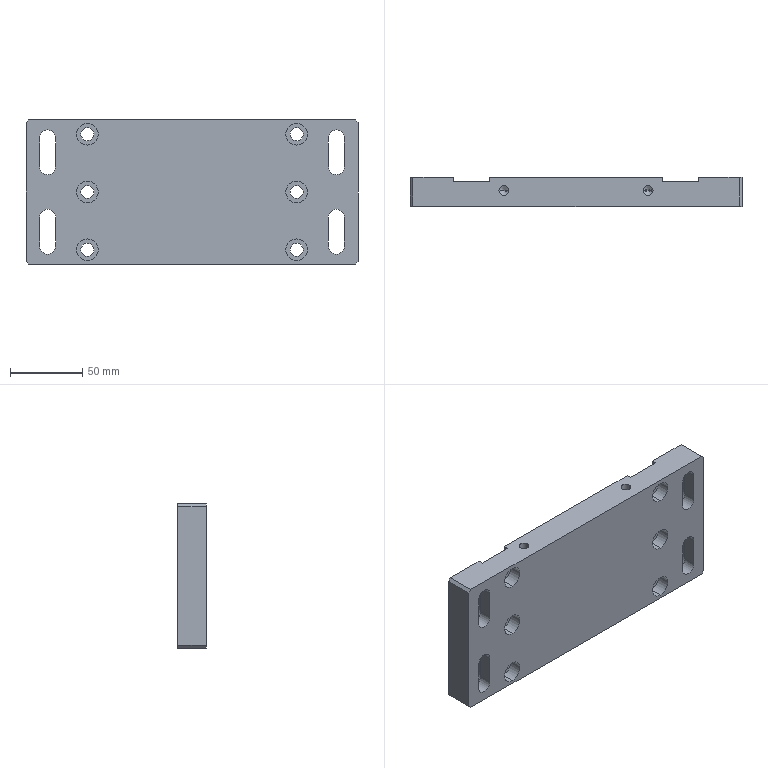Part | SolidWorks | features HoleWzd 3, Chamfer 1, Extrusion 1, ICE 1 | 1 solid | 100 faces | box 230 x 20 x 100 mm | volume 391656 mm3 | cylinder 52 | plane 44 | cone 4 | commonest cylinder face diameters 9 x12 11 x12 15 x12 18 x12 6.8 x4